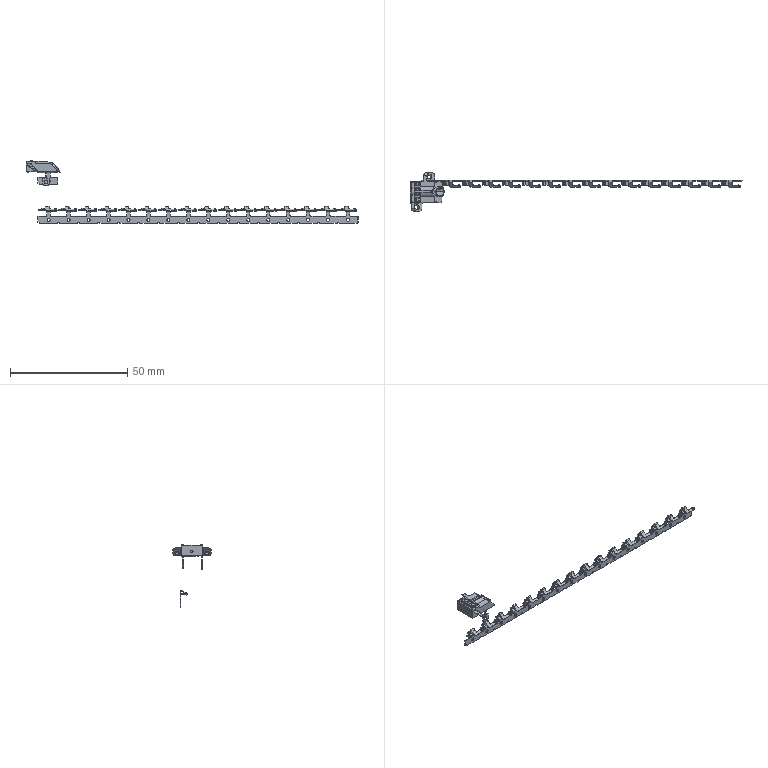Part | NX | 6 solids | 2736 faces | box 141.41 x 16.558 x 26.718 mm | volume 490.865 mm3 | plane 1270 | cylinder 960 | torus 346 | sphere 120 | spline 22 | cone 18 | commonest cylinder face diameters 0.2 x235 0.4 x143 0.5 x113 0.7 x86 1 x67 0.6 x61